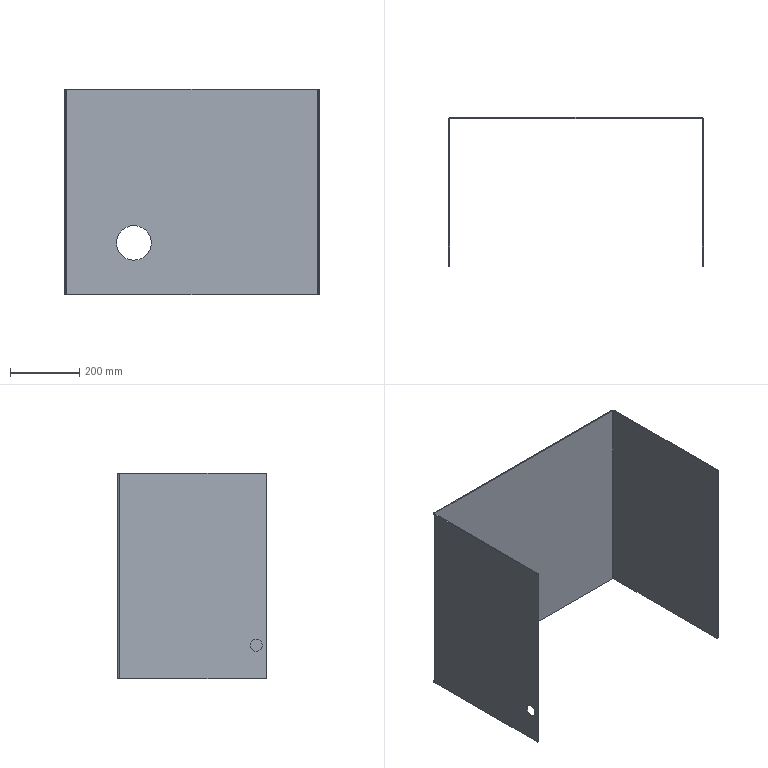Part | SolidWorks | features ICE 3, FlatPattern 1, SMBaseFlange 1, SheetMetal 1 | 1 solid | 30 faces | box 736 x 430 x 594 mm | volume 2800017 mm3 | plane 18 | cylinder 12 | commonest cylinder face diameters 7 x4 6 x2 12 x2 35 x2 100 x2
STEP:
#1=CARTESIAN_POINT('',(200.,427.,100.));
#2=VERTEX_POINT('',#1);
#3=CARTESIAN_POINT('',(200.,427.,200.));
#4=VERTEX_POINT('',#3);
#5=CARTESIAN_POINT('',(200.,427.,150.));
#6=DIRECTION('',(0.,1.,0.));
#7=DIRECTION('',(0.,0.,1.));
#8=AXIS2_PLACEMENT_3D('',#5,#6,#7);
#9=CIRCLE('',#8,50.);
#10=EDGE_CURVE('',#2,#4,#9,.T.);
#11=ORIENTED_EDGE('',*,*,#10,.F.);
#12=CARTESIAN_POINT('',(200.,430.,100.));
#13=VERTEX_POINT('',#12);
#14=CARTESIAN_POINT('',(200.,420.,100.));
#15=DIRECTION('',(0.,1.,0.));
#16=VECTOR('',#15,1000.);
#17=LINE('',#14,#16);
#18=EDGE_CURVE('',#2,#13,#17,.T.);
#19=ORIENTED_EDGE('',*,*,#18,.T.);
#20=CARTESIAN_POINT('',(200.,430.,200.));
#21=VERTEX_POINT('',#20);
#22=CARTESIAN_POINT('',(200.,430.,150.));
#23=DIRECTION('',(0.,1.,0.));
#24=DIRECTION('',(0.,0.,1.));
#25=AXIS2_PLACEMENT_3D('',#22,#23,#24);
#26=CIRCLE('',#25,50.);
#27=EDGE_CURVE('',#13,#21,#26,.T.);
#28=ORIENTED_EDGE('',*,*,#27,.T.);
#29=CARTESIAN_POINT('',(200.,420.,200.));
#30=DIRECTION('',(0.,1.,0.));
#31=VECTOR('',#30,1000.);
#32=LINE('',#29,#31);
#33=EDGE_CURVE('',#4,#21,#32,.T.);
#34=ORIENTED_EDGE('',*,*,#33,.F.);
#35=EDGE_LOOP('',(#11,#19,#28,#34));
#36=FACE_OUTER_BOUND('',#35,.T.);
#37=CARTESIAN_POINT('',(200.,420.,150.));
#38=DIRECTION('',(0.,1.,0.));
#39=DIRECTION('',(0.,0.,1.));
#40=AXIS2_PLACEMENT_3D('',#37,#38,#39);
#41=CYLINDRICAL_SURFACE('',#40,50.);
#42=ADVANCED_FACE('',(#36),#41,.F.);
#43=CARTESIAN_POINT('',(3.,30.,79.5));
#44=VERTEX_POINT('',#43);
#45=CARTESIAN_POINT('',(3.,30.,114.5));
#46=VERTEX_POINT('',#45);
#47=CARTESIAN_POINT('',(3.,30.,97.));
#48=DIRECTION('',(-1.,0.,0.));
#49=DIRECTION('',(0.,0.,1.));
#50=AXIS2_PLACEMENT_3D('',#47,#48,#49);
#51=CIRCLE('',#50,17.5);
#52=EDGE_CURVE('',#44,#46,#51,.T.);
#53=ORIENTED_EDGE('',*,*,#52,.F.);
#54=CARTESIAN_POINT('',(0.,30.,79.5));
#55=VERTEX_POINT('',#54);
#56=CARTESIAN_POINT('',(10.,30.,79.5));
#57=DIRECTION('',(-1.,0.,0.));
#58=VECTOR('',#57,1000.);
#59=LINE('',#56,#58);
#60=EDGE_CURVE('',#44,#55,#59,.T.);
#61=ORIENTED_EDGE('',*,*,#60,.T.);
#62=CARTESIAN_POINT('',(0.,30.,114.5));
#63=VERTEX_POINT('',#62);
#64=CARTESIAN_POINT('',(0.,30.,97.));
#65=DIRECTION('',(-1.,0.,0.));
#66=DIRECTION('',(0.,0.,1.));
#67=AXIS2_PLACEMENT_3D('',#64,#65,#66);
#68=CIRCLE('',#67,17.5);
#69=EDGE_CURVE('',#55,#63,#68,.T.);
#70=ORIENTED_EDGE('',*,*,#69,.T.);
#71=CARTESIAN_POINT('',(10.,30.,114.5));
#72=DIRECTION('',(-1.,0.,0.));
#73=VECTOR('',#72,1000.);
#74=LINE('',#71,#73);
#75=EDGE_CURVE('',#46,#63,#74,.T.);
#76=ORIENTED_EDGE('',*,*,#75,.F.);
#77=EDGE_LOOP('',(#53,#61,#70,#76));
#78=FACE_OUTER_BOUND('',#77,.T.);
#79=CARTESIAN_POINT('',(10.,30.,97.));
#80=DIRECTION('',(-1.,0.,0.));
#81=DIRECTION('',(0.,0.,1.));
#82=AXIS2_PLACEMENT_3D('',#79,#80,#81);
#83=CYLINDRICAL_SURFACE('',#82,17.5);
#84=ADVANCED_FACE('',(#78),#83,.F.);
#85=CARTESIAN_POINT('',(733.,0.,590.5));
#86=VERTEX_POINT('',#85);
#87=CARTESIAN_POINT('',(733.,3.5,594.));
#88=VERTEX_POINT('',#87);
#89=CARTESIAN_POINT('',(733.,3.5,590.5));
#90=DIRECTION('',(-1.,0.,0.));
#91=DIRECTION('',(0.,0.,-1.));
#92=AXIS2_PLACEMENT_3D('',#89,#90,#91);
#93=CIRCLE('',#92,3.5);
#94=EDGE_CURVE('',#86,#88,#93,.T.);
#95=ORIENTED_EDGE('',*,*,#94,.T.);
#96=CARTESIAN_POINT('',(733.,424.,594.));
#97=VERTEX_POINT('',#96);
#98=CARTESIAN_POINT('',(733.,430.,594.));
#99=DIRECTION('',(0.,-1.,0.));
#100=VECTOR('',#99,1000.);
#101=LINE('',#98,#100);
#102=EDGE_CURVE('',#97,#88,#101,.T.);
#103=ORIENTED_EDGE('',*,*,#102,.F.);
#104=CARTESIAN_POINT('',(733.,424.,0.));
#105=VERTEX_POINT('',#104);
#106=CARTESIAN_POINT('',(733.,424.,594.));
#107=DIRECTION('',(0.,0.,-1.));
#108=VECTOR('',#107,1000.);
#109=LINE('',#106,#108);
#110=EDGE_CURVE('',#97,#105,#109,.T.);
#111=ORIENTED_EDGE('',*,*,#110,.T.);
#112=CARTESIAN_POINT('',(733.,3.5,0.));
#113=VERTEX_POINT('',#112);
#114=CARTESIAN_POINT('',(733.,430.,0.));
#115=DIRECTION('',(0.,-1.,0.));
#116=VECTOR('',#115,1000.);
#117=LINE('',#114,#116);
#118=EDGE_CURVE('',#105,#113,#117,.T.);
#119=ORIENTED_EDGE('',*,*,#118,.T.);
#120=CARTESIAN_POINT('',(733.,0.,3.5));
#121=VERTEX_POINT('',#120);
#122=CARTESIAN_POINT('',(733.,3.5,3.5));
#123=DIRECTION('',(-1.,0.,0.));
#124=DIRECTION('',(0.,0.,-1.));
#125=AXIS2_PLACEMENT_3D('',#122,#123,#124);
#126=CIRCLE('',#125,3.5);
#127=EDGE_CURVE('',#113,#121,#126,.T.);
#128=ORIENTED_EDGE('',*,*,#127,.T.);
#129=CARTESIAN_POINT('',(733.,0.,594.));
#130=DIRECTION('',(0.,0.,-1.));
#131=VECTOR('',#130,1000.);
#132=LINE('',#129,#131);
#133=EDGE_CURVE('',#86,#121,#132,.T.);
#134=ORIENTED_EDGE('',*,*,#133,.F.);
#135=EDGE_LOOP('',(#95,#103,#111,#119,#128,#134));
#136=FACE_OUTER_BOUND('',#135,.T.);
#137=CARTESIAN_POINT('',(733.,430.,594.));
#138=DIRECTION('',(1.,0.,0.));
#139=DIRECTION('',(0.,0.,-1.));
#140=AXIS2_PLACEMENT_3D('',#137,#138,#139);
#141=PLANE('',#140);
#142=ADVANCED_FACE('',(#136),#141,.F.);
#143=CARTESIAN_POINT('',(736.,424.,594.));
#144=VERTEX_POINT('',#143);
#145=CARTESIAN_POINT('',(736.,3.5,594.));
#146=VERTEX_POINT('',#145);
#147=CARTESIAN_POINT('',(736.,430.,594.));
#148=DIRECTION('',(0.,-1.,0.));
#149=VECTOR('',#148,1000.);
#150=LINE('',#147,#149);
#151=EDGE_CURVE('',#144,#146,#150,.T.);
#152=ORIENTED_EDGE('',*,*,#151,.T.);
#153=CARTESIAN_POINT('',(736.,0.,590.5));
#154=VERTEX_POINT('',#153);
#155=CARTESIAN_POINT('',(736.,3.5,590.5));
#156=DIRECTION('',(-1.,0.,0.));
#157=DIRECTION('',(0.,0.,-1.));
#158=AXIS2_PLACEMENT_3D('',#155,#156,#157);
#159=CIRCLE('',#158,3.5);
#160=EDGE_CURVE('',#154,#146,#159,.T.);
#161=ORIENTED_EDGE('',*,*,#160,.F.);
#162=CARTESIAN_POINT('',(736.,0.,3.5));
#163=VERTEX_POINT('',#162);
#164=CARTESIAN_POINT('',(736.,0.,594.));
#165=DIRECTION('',(0.,0.,-1.));
#166=VECTOR('',#165,1000.);
#167=LINE('',#164,#166);
#168=EDGE_CURVE('',#154,#163,#167,.T.);
#169=ORIENTED_EDGE('',*,*,#168,.T.);
#170=CARTESIAN_POINT('',(736.,3.5,0.));
#171=VERTEX_POINT('',#170);
#172=CARTESIAN_POINT('',(736.,3.5,3.5));
#173=DIRECTION('',(-1.,0.,0.));
#174=DIRECTION('',(0.,0.,-1.));
#175=AXIS2_PLACEMENT_3D('',#172,#173,#174);
#176=CIRCLE('',#175,3.5);
#177=EDGE_CURVE('',#171,#163,#176,.T.);
#178=ORIENTED_EDGE('',*,*,#177,.F.);
#179=CARTESIAN_POINT('',(736.,424.,0.));
#180=VERTEX_POINT('',#179);
#181=CARTESIAN_POINT('',(736.,430.,0.));
#182=DIRECTION('',(0.,-1.,0.));
#183=VECTOR('',#182,1000.);
#184=LINE('',#181,#183);
#185=EDGE_CURVE('',#180,#171,#184,.T.);
#186=ORIENTED_EDGE('',*,*,#185,.F.);
#187=CARTESIAN_POINT('',(736.,424.,594.));
#188=DIRECTION('',(0.,0.,-1.));
#189=VECTOR('',#188,1000.);
#190=LINE('',#187,#189);
#191=EDGE_CURVE('',#144,#180,#190,.T.);
#192=ORIENTED_EDGE('',*,*,#191,.F.);
#193=EDGE_LOOP('',(#152,#161,#169,#178,#186,#192));
#194=FACE_OUTER_BOUND('',#193,.T.);
#195=CARTESIAN_POINT('',(736.,430.,594.));
#196=DIRECTION('',(1.,0.,0.));
#197=DIRECTION('',(0.,0.,-1.));
#198=AXIS2_PLACEMENT_3D('',#195,#196,#197);
#199=PLANE('',#198);
#200=ADVANCED_FACE('',(#194),#199,.T.);
#201=ORIENTED_EDGE('',*,*,#102,.T.);
#202=CARTESIAN_POINT('',(733.,3.5,594.));
#203=DIRECTION('',(1.,0.,0.));
#204=VECTOR('',#203,1000.);
#205=LINE('',#202,#204);
#206=EDGE_CURVE('',#88,#146,#205,.T.);
#207=ORIENTED_EDGE('',*,*,#206,.T.);
#208=ORIENTED_EDGE('',*,*,#151,.F.);
#209=CARTESIAN_POINT('',(736.,424.,594.));
#210=DIRECTION('',(-1.,0.,0.));
#211=VECTOR('',#210,1000.);
#212=LINE('',#209,#211);
#213=EDGE_CURVE('',#144,#97,#212,.T.);
#214=ORIENTED_EDGE('',*,*,#213,.T.);
#215=EDGE_LOOP('',(#201,#207,#208,#214));
#216=FACE_OUTER_BOUND('',#215,.T.);
#217=CARTESIAN_POINT('',(730.,427.,594.));
#218=DIRECTION('',(0.,0.,1.));
#219=DIRECTION('',(1.,0.,0.));
#220=AXIS2_PLACEMENT_3D('',#217,#218,#219);
#221=PLANE('',#220);
#222=ADVANCED_FACE('',(#216),#221,.T.);
#223=CARTESIAN_POINT('',(733.,0.,590.5));
#224=DIRECTION('',(1.,0.,0.));
#225=VECTOR('',#224,1000.);
#226=LINE('',#223,#225);
#227=EDGE_CURVE('',#86,#154,#226,.T.);
#228=ORIENTED_EDGE('',*,*,#227,.F.);
#229=ORIENTED_EDGE('',*,*,#133,.T.);
#230=CARTESIAN_POINT('',(733.,0.,3.5));
#231=DIRECTION('',(1.,0.,0.));
#232=VECTOR('',#231,1000.);
#233=LINE('',#230,#232);
#234=EDGE_CURVE('',#121,#163,#233,.T.);
#235=ORIENTED_EDGE('',*,*,#234,.T.);
#236=ORIENTED_EDGE('',*,*,#168,.F.);
#237=EDGE_LOOP('',(#228,#229,#235,#236));
#238=FACE_OUTER_BOUND('',#237,.T.);
#239=CARTESIAN_POINT('',(736.,0.,594.));
#240=DIRECTION('',(0.,-1.,0.));
#241=DIRECTION('',(0.,0.,-1.));
#242=AXIS2_PLACEMENT_3D('',#239,#240,#241);
#243=PLANE('',#242);
#244=ADVANCED_FACE('',(#238),#243,.T.);
#245=CARTESIAN_POINT('',(733.,3.5,0.));
#246=DIRECTION('',(1.,0.,0.));
#247=VECTOR('',#246,1000.);
#248=LINE('',#245,#247);
#249=EDGE_CURVE('',#113,#171,#248,.T.);
#250=ORIENTED_EDGE('',*,*,#249,.F.);
#251=ORIENTED_EDGE('',*,*,#118,.F.);
#252=CARTESIAN_POINT('',(733.,424.,0.));
#253=DIRECTION('',(1.,0.,0.));
#254=VECTOR('',#253,1000.);
#255=LINE('',#252,#254);
#256=EDGE_CURVE('',#105,#180,#255,.T.);
#257=ORIENTED_EDGE('',*,*,#256,.T.);
#258=ORIENTED_EDGE('',*,*,#185,.T.);
#259=EDGE_LOOP('',(#250,#251,#257,#258));
#260=FACE_OUTER_BOUND('',#259,.T.);
#261=CARTESIAN_POINT('',(730.,424.,0.));
#262=DIRECTION('',(0.,0.,1.));
#263=DIRECTION('',(1.,0.,0.));
#264=AXIS2_PLACEMENT_3D('',#261,#262,#263);
#265=PLANE('',#264);
#266=ADVANCED_FACE('',(#260),#265,.F.);
#267=CARTESIAN_POINT('',(0.,30.,97.));
#268=DIRECTION('',(-1.,0.,0.));
#269=DIRECTION('',(0.,0.,1.));
#270=AXIS2_PLACEMENT_3D('',#267,#268,#269);
#271=CIRCLE('',#270,17.5);
#272=EDGE_CURVE('',#63,#55,#271,.T.);
#273=ORIENTED_EDGE('',*,*,#272,.F.);
#274=ORIENTED_EDGE('',*,*,#69,.F.);
#275=EDGE_LOOP('',(#273,#274));
#276=FACE_BOUND('',#275,.T.);
#277=CARTESIAN_POINT('',(0.,0.,590.5));
#278=VERTEX_POINT('',#277);
#279=CARTESIAN_POINT('',(0.,0.,3.5));
#280=VERTEX_POINT('',#279);
#281=CARTESIAN_POINT('',(0.,0.,594.));
#282=DIRECTION('',(0.,0.,-1.));
#283=VECTOR('',#282,1000.);
#284=LINE('',#281,#283);
#285=EDGE_CURVE('',#278,#280,#284,.T.);
#286=ORIENTED_EDGE('',*,*,#285,.F.);
#287=CARTESIAN_POINT('',(0.,3.5,594.));
#288=VERTEX_POINT('',#287);
#289=CARTESIAN_POINT('',(0.,3.5,590.5));
#290=DIRECTION('',(1.,0.,0.));
#291=DIRECTION('',(0.,0.,1.));
#292=AXIS2_PLACEMENT_3D('',#289,#290,#291);
#293=CIRCLE('',#292,3.5);
#294=EDGE_CURVE('',#288,#278,#293,.T.);
#295=ORIENTED_EDGE('',*,*,#294,.F.);
#296=CARTESIAN_POINT('',(0.,424.,594.));
#297=VERTEX_POINT('',#296);
#298=CARTESIAN_POINT('',(0.,0.,594.));
#299=DIRECTION('',(0.,1.,0.));
#300=VECTOR('',#299,1000.);
#301=LINE('',#298,#300);
#302=EDGE_CURVE('',#288,#297,#301,.T.);
#303=ORIENTED_EDGE('',*,*,#302,.T.);
#304=CARTESIAN_POINT('',(0.,424.,0.));
#305=VERTEX_POINT('',#304);
#306=CARTESIAN_POINT('',(0.,424.,594.));
#307=DIRECTION('',(0.,0.,-1.));
#308=VECTOR('',#307,1000.);
#309=LINE('',#306,#308);
#310=EDGE_CURVE('',#297,#305,#309,.T.);
#311=ORIENTED_EDGE('',*,*,#310,.T.);
#312=CARTESIAN_POINT('',(0.,3.5,0.));
#313=VERTEX_POINT('',#312);
#314=CARTESIAN_POINT('',(0.,0.,0.));
#315=DIRECTION('',(0.,1.,0.));
#316=VECTOR('',#315,1000.);
#317=LINE('',#314,#316);
#318=EDGE_CURVE('',#313,#305,#317,.T.);
#319=ORIENTED_EDGE('',*,*,#318,.F.);
#320=CARTESIAN_POINT('',(0.,3.5,3.5));
#321=DIRECTION('',(1.,0.,0.));
#322=DIRECTION('',(0.,0.,1.));
#323=AXIS2_PLACEMENT_3D('',#320,#321,#322);
#324=CIRCLE('',#323,3.5);
#325=EDGE_CURVE('',#280,#313,#324,.T.);
#326=ORIENTED_EDGE('',*,*,#325,.F.);
#327=EDGE_LOOP('',(#286,#295,#303,#311,#319,#326));
#328=FACE_OUTER_BOUND('',#327,.T.);
#329=CARTESIAN_POINT('',(0.,0.,594.));
#330=DIRECTION('',(-1.,0.,0.));
#331=DIRECTION('',(0.,0.,1.));
#332=AXIS2_PLACEMENT_3D('',#329,#330,#331);
#333=PLANE('',#332);
#334=ADVANCED_FACE('',(#276,#328),#333,.T.);
#335=CARTESIAN_POINT('',(3.,30.,97.));
#336=DIRECTION('',(-1.,0.,0.));
#337=DIRECTION('',(0.,0.,1.));
#338=AXIS2_PLACEMENT_3D('',#335,#336,#337);
#339=CIRCLE('',#338,17.5);
#340=EDGE_CURVE('',#46,#44,#339,.T.);
#341=ORIENTED_EDGE('',*,*,#340,.T.);
#342=ORIENTED_EDGE('',*,*,#52,.T.);
#343=EDGE_LOOP('',(#341,#342));
#344=FACE_BOUND('',#343,.T.);
#345=CARTESIAN_POINT('',(3.,3.5,594.));
#346=VERTEX_POINT('',#345);
#347=CARTESIAN_POINT('',(3.,0.,590.5));
#348=VERTEX_POINT('',#347);
#349=CARTESIAN_POINT('',(3.,3.5,590.5));
#350=DIRECTION('',(1.,0.,0.));
#351=DIRECTION('',(0.,0.,1.));
#352=AXIS2_PLACEMENT_3D('',#349,#350,#351);
#353=CIRCLE('',#352,3.5);
#354=EDGE_CURVE('',#346,#348,#353,.T.);
#355=ORIENTED_EDGE('',*,*,#354,.T.);
#356=CARTESIAN_POINT('',(3.,0.,3.5));
#357=VERTEX_POINT('',#356);
#358=CARTESIAN_POINT('',(3.,0.,594.));
#359=DIRECTION('',(0.,0.,-1.));
#360=VECTOR('',#359,1000.);
#361=LINE('',#358,#360);
#362=EDGE_CURVE('',#348,#357,#361,.T.);
#363=ORIENTED_EDGE('',*,*,#362,.T.);
#364=CARTESIAN_POINT('',(3.,3.5,0.));
#365=VERTEX_POINT('',#364);
#366=CARTESIAN_POINT('',(3.,3.5,3.5));
#367=DIRECTION('',(1.,0.,0.));
#368=DIRECTION('',(0.,0.,1.));
#369=AXIS2_PLACEMENT_3D('',#366,#367,#368);
#370=CIRCLE('',#369,3.5);
#371=EDGE_CURVE('',#357,#365,#370,.T.);
#372=ORIENTED_EDGE('',*,*,#371,.T.);
#373=CARTESIAN_POINT('',(3.,424.,0.));
#374=VERTEX_POINT('',#373);
#375=CARTESIAN_POINT('',(3.,0.,0.));
#376=DIRECTION('',(0.,1.,0.));
#377=VECTOR('',#376,1000.);
#378=LINE('',#375,#377);
#379=EDGE_CURVE('',#365,#374,#378,.T.);
#380=ORIENTED_EDGE('',*,*,#379,.T.);
#381=CARTESIAN_POINT('',(3.,424.,594.));
#382=VERTEX_POINT('',#381);
#383=CARTESIAN_POINT('',(3.,424.,594.));
#384=DIRECTION('',(0.,0.,-1.));
#385=VECTOR('',#384,1000.);
#386=LINE('',#383,#385);
#387=EDGE_CURVE('',#382,#374,#386,.T.);
#388=ORIENTED_EDGE('',*,*,#387,.F.);
#389=CARTESIAN_POINT('',(3.,0.,594.));
#390=DIRECTION('',(0.,1.,0.));
#391=VECTOR('',#390,1000.);
#392=LINE('',#389,#391);
#393=EDGE_CURVE('',#346,#382,#392,.T.);
#394=ORIENTED_EDGE('',*,*,#393,.F.);
#395=EDGE_LOOP('',(#355,#363,#372,#380,#388,#394));
#396=FACE_OUTER_BOUND('',#395,.T.);
#397=CARTESIAN_POINT('',(3.,0.,594.));
#398=DIRECTION('',(-1.,0.,0.));
#399=DIRECTION('',(0.,0.,1.));
#400=AXIS2_PLACEMENT_3D('',#397,#398,#399);
#401=PLANE('',#400);
#402=ADVANCED_FACE('',(#344,#396),#401,.F.);
#403=ORIENTED_EDGE('',*,*,#362,.F.);
#404=CARTESIAN_POINT('',(3.,0.,590.5));
#405=DIRECTION('',(-1.,0.,0.));
#406=VECTOR('',#405,1000.);
#407=LINE('',#404,#406);
#408=EDGE_CURVE('',#348,#278,#407,.T.);
#409=ORIENTED_EDGE('',*,*,#408,.T.);
#410=ORIENTED_EDGE('',*,*,#285,.T.);
#411=CARTESIAN_POINT('',(3.,0.,3.5));
#412=DIRECTION('',(-1.,0.,0.));
#413=VECTOR('',#412,1000.);
#414=LINE('',#411,#413);
#415=EDGE_CURVE('',#357,#280,#414,.T.);
#416=ORIENTED_EDGE('',*,*,#415,.F.);
#417=EDGE_LOOP('',(#403,#409,#410,#416));
#418=FACE_OUTER_BOUND('',#417,.T.);
#419=CARTESIAN_POINT('',(3.,0.,594.));
#420=DIRECTION('',(0.,-1.,0.));
#421=DIRECTION('',(0.,0.,-1.));
#422=AXIS2_PLACEMENT_3D('',#419,#420,#421);
#423=PLANE('',#422);
#424=ADVANCED_FACE('',(#418),#423,.T.);
#425=ORIENTED_EDGE('',*,*,#379,.F.);
#426=CARTESIAN_POINT('',(3.,3.5,0.));
#427=DIRECTION('',(-1.,0.,0.));
#428=VECTOR('',#427,1000.);
#429=LINE('',#426,#428);
#430=EDGE_CURVE('',#365,#313,#429,.T.);
#431=ORIENTED_EDGE('',*,*,#430,.T.);
#432=ORIENTED_EDGE('',*,*,#318,.T.);
#433=CARTESIAN_POINT('',(0.,424.,0.));
#434=DIRECTION('',(1.,0.,0.));
#435=VECTOR('',#434,1000.);
#436=LINE('',#433,#435);
#437=EDGE_CURVE('',#305,#374,#436,.T.);
#438=ORIENTED_EDGE('',*,*,#437,.T.);
#439=EDGE_LOOP('',(#425,#431,#432,#438));
#440=FACE_OUTER_BOUND('',#439,.T.);
#441=CARTESIAN_POINT('',(6.,427.,0.));
#442=DIRECTION('',(0.,0.,-1.));
#443=DIRECTION('',(-1.,0.,0.));
#444=AXIS2_PLACEMENT_3D('',#441,#442,#443);
#445=PLANE('',#444);
#446=ADVANCED_FACE('',(#440),#445,.T.);
#447=CARTESIAN_POINT('',(6.,430.,594.));
#448=VERTEX_POINT('',#447);
#449=CARTESIAN_POINT('',(6.,427.,594.));
#450=VERTEX_POINT('',#449);
#451=CARTESIAN_POINT('',(6.,430.,594.));
#452=DIRECTION('',(0.,-1.,0.));
#453=VECTOR('',#452,1000.);
#454=LINE('',#451,#453);
#455=EDGE_CURVE('',#448,#450,#454,.T.);
#456=ORIENTED_EDGE('',*,*,#455,.F.);
#457=CARTESIAN_POINT('',(6.,424.,594.));
#458=DIRECTION('',(0.,0.,-1.));
#459=DIRECTION('',(1.,0.,0.));
#460=AXIS2_PLACEMENT_3D('',#457,#458,#459);
#461=CIRCLE('',#460,6.);
#462=EDGE_CURVE('',#297,#448,#461,.T.);
#463=ORIENTED_EDGE('',*,*,#462,.F.);
#464=CARTESIAN_POINT('',(3.,424.,594.));
#465=DIRECTION('',(-1.,0.,0.));
#466=VECTOR('',#465,1000.);
#467=LINE('',#464,#466);
#468=EDGE_CURVE('',#382,#297,#467,.T.);
#469=ORIENTED_EDGE('',*,*,#468,.F.);
#470=CARTESIAN_POINT('',(6.,424.,594.));
#471=DIRECTION('',(0.,0.,-1.));
#472=DIRECTION('',(1.,0.,0.));
#473=AXIS2_PLACEMENT_3D('',#470,#471,#472);
#474=CIRCLE('',#473,3.);
#475=EDGE_CURVE('',#382,#450,#474,.T.);
#476=ORIENTED_EDGE('',*,*,#475,.T.);
#477=EDGE_LOOP('',(#456,#463,#469,#476));
#478=FACE_OUTER_BOUND('',#477,.T.);
#479=CARTESIAN_POINT('',(6.,430.,594.));
#480=DIRECTION('',(0.,0.,1.));
#481=DIRECTION('',(1.,0.,0.));
#482=AXIS2_PLACEMENT_3D('',#479,#480,#481);
#483=PLANE('',#482);
#484=ADVANCED_FACE('',(#478),#483,.T.);
#485=CARTESIAN_POINT('',(730.,430.,594.));
#486=VERTEX_POINT('',#485);
#487=CARTESIAN_POINT('',(0.,430.,594.));
#488=DIRECTION('',(1.,0.,0.));
#489=VECTOR('',#488,1000.);
#490=LINE('',#487,#489);
#491=EDGE_CURVE('',#448,#486,#490,.T.);
#492=ORIENTED_EDGE('',*,*,#491,.F.);
#493=ORIENTED_EDGE('',*,*,#455,.T.);
#494=CARTESIAN_POINT('',(730.,427.,594.));
#495=VERTEX_POINT('',#494);
#496=CARTESIAN_POINT('',(0.,427.,594.));
#497=DIRECTION('',(1.,0.,0.));
#498=VECTOR('',#497,1000.);
#499=LINE('',#496,#498);
#500=EDGE_CURVE('',#450,#495,#499,.T.);
#501=ORIENTED_EDGE('',*,*,#500,.T.);
#502=CARTESIAN_POINT('',(730.,427.,594.));
#503=DIRECTION('',(0.,1.,0.));
#504=VECTOR('',#503,1000.);
#505=LINE('',#502,#504);
#506=EDGE_CURVE('',#495,#486,#505,.T.);
#507=ORIENTED_EDGE('',*,*,#506,.T.);
#508=EDGE_LOOP('',(#492,#493,#501,#507));
#509=FACE_OUTER_BOUND('',#508,.T.);
#510=CARTESIAN_POINT('',(3.,424.,594.));
#511=DIRECTION('',(0.,0.,1.));
#512=DIRECTION('',(1.,0.,0.));
#513=AXIS2_PLACEMENT_3D('',#510,#511,#512);
#514=PLANE('',#513);
#515=ADVANCED_FACE('',(#509),#514,.T.);
#516=ORIENTED_EDGE('',*,*,#437,.F.);
#517=CARTESIAN_POINT('',(6.,430.,0.));
#518=VERTEX_POINT('',#517);
#519=CARTESIAN_POINT('',(6.,424.,0.));
#520=DIRECTION('',(0.,0.,-1.));
#521=DIRECTION('',(1.,0.,0.));
#522=AXIS2_PLACEMENT_3D('',#519,#520,#521);
#523=CIRCLE('',#522,6.);
#524=EDGE_CURVE('',#305,#518,#523,.T.);
#525=ORIENTED_EDGE('',*,*,#524,.T.);
#526=CARTESIAN_POINT('',(6.,427.,0.));
#527=VERTEX_POINT('',#526);
#528=CARTESIAN_POINT('',(6.,427.,0.));
#529=DIRECTION('',(0.,1.,0.));
#530=VECTOR('',#529,1000.);
#531=LINE('',#528,#530);
#532=EDGE_CURVE('',#527,#518,#531,.T.);
#533=ORIENTED_EDGE('',*,*,#532,.F.);
#534=CARTESIAN_POINT('',(6.,424.,0.));
#535=DIRECTION('',(0.,0.,-1.));
#536=DIRECTION('',(1.,0.,0.));
#537=AXIS2_PLACEMENT_3D('',#534,#535,#536);
#538=CIRCLE('',#537,3.);
#539=EDGE_CURVE('',#374,#527,#538,.T.);
#540=ORIENTED_EDGE('',*,*,#539,.F.);
#541=EDGE_LOOP('',(#516,#525,#533,#540));
#542=FACE_OUTER_BOUND('',#541,.T.);
#543=CARTESIAN_POINT('',(0.,424.,0.));
#544=DIRECTION('',(0.,0.,-1.));
#545=DIRECTION('',(-1.,0.,0.));
#546=AXIS2_PLACEMENT_3D('',#543,#544,#545);
#547=PLANE('',#546);
#548=ADVANCED_FACE('',(#542),#547,.T.);
#549=ORIENTED_EDGE('',*,*,#213,.F.);
#550=CARTESIAN_POINT('',(730.,424.,594.));
#551=DIRECTION('',(0.,0.,-1.));
#552=DIRECTION('',(1.,0.,0.));
#553=AXIS2_PLACEMENT_3D('',#550,#551,#552);
#554=CIRCLE('',#553,6.);
#555=EDGE_CURVE('',#486,#144,#554,.T.);
#556=ORIENTED_EDGE('',*,*,#555,.F.);
#557=ORIENTED_EDGE('',*,*,#506,.F.);
#558=CARTESIAN_POINT('',(730.,424.,594.));
#559=DIRECTION('',(0.,0.,-1.));
#560=DIRECTION('',(1.,0.,0.));
#561=AXIS2_PLACEMENT_3D('',#558,#559,#560);
#562=CIRCLE('',#561,3.);
#563=EDGE_CURVE('',#495,#97,#562,.T.);
#564=ORIENTED_EDGE('',*,*,#563,.T.);
#565=EDGE_LOOP('',(#549,#556,#557,#564));
#566=FACE_OUTER_BOUND('',#565,.T.);
#567=CARTESIAN_POINT('',(736.,424.,594.));
#568=DIRECTION('',(0.,0.,1.));
#569=DIRECTION('',(1.,0.,0.));
#570=AXIS2_PLACEMENT_3D('',#567,#568,#569);
#571=PLANE('',#570);
#572=ADVANCED_FACE('',(#566),#571,.T.);
#573=CARTESIAN_POINT('',(730.,430.,0.));
#574=VERTEX_POINT('',#573);
#575=CARTESIAN_POINT('',(730.,427.,0.));
#576=VERTEX_POINT('',#575);
#577=CARTESIAN_POINT('',(730.,430.,0.));
#578=DIRECTION('',(0.,-1.,0.));
#579=VECTOR('',#578,1000.);
#580=LINE('',#577,#579);
#581=EDGE_CURVE('',#574,#576,#580,.T.);
#582=ORIENTED_EDGE('',*,*,#581,.F.);
#583=CARTESIAN_POINT('',(730.,424.,0.));
#584=DIRECTION('',(0.,0.,-1.));
#585=DIRECTION('',(1.,0.,0.));
#586=AXIS2_PLACEMENT_3D('',#583,#584,#585);
#587=CIRCLE('',#586,6.);
#588=EDGE_CURVE('',#574,#180,#587,.T.);
#589=ORIENTED_EDGE('',*,*,#588,.T.);
#590=ORIENTED_EDGE('',*,*,#256,.F.);
#591=CARTESIAN_POINT('',(730.,424.,0.));
#592=DIRECTION('',(0.,0.,-1.));
#593=DIRECTION('',(1.,0.,0.));
#594=AXIS2_PLACEMENT_3D('',#591,#592,#593);
#595=CIRCLE('',#594,3.);
#596=EDGE_CURVE('',#576,#105,#595,.T.);
#597=ORIENTED_EDGE('',*,*,#596,.F.);
#598=EDGE_LOOP('',(#582,#589,#590,#597));
#599=FACE_OUTER_BOUND('',#598,.T.);
#600=CARTESIAN_POINT('',(730.,430.,0.));
#601=DIRECTION('',(0.,0.,-1.));
#602=DIRECTION('',(-1.,0.,0.));
#603=AXIS2_PLACEMENT_3D('',#600,#601,#602);
#604=PLANE('',#603);
#605=ADVANCED_FACE('',(#599),#604,.T.);
#606=CARTESIAN_POINT('',(0.,430.,0.));
#607=DIRECTION('',(1.,0.,0.));
#608=VECTOR('',#607,1000.);
#609=LINE('',#606,#608);
#610=EDGE_CURVE('',#518,#574,#609,.T.);
#611=ORIENTED_EDGE('',*,*,#610,.T.);
#612=ORIENTED_EDGE('',*,*,#581,.T.);
#613=CARTESIAN_POINT('',(0.,427.,0.));
#614=DIRECTION('',(1.,0.,0.));
#615=VECTOR('',#614,1000.);
#616=LINE('',#613,#615);
#617=EDGE_CURVE('',#527,#576,#616,.T.);
#618=ORIENTED_EDGE('',*,*,#617,.F.);
#619=ORIENTED_EDGE('',*,*,#532,.T.);
#620=EDGE_LOOP('',(#611,#612,#618,#619));
#621=FACE_OUTER_BOUND('',#620,.T.);
#622=CARTESIAN_POINT('',(733.,424.,0.));
#623=DIRECTION('',(0.,0.,-1.));
#624=DIRECTION('',(-1.,0.,0.));
#625=AXIS2_PLACEMENT_3D('',#622,#623,#624);
#626=PLANE('',#625);
#627=ADVANCED_FACE('',(#621),#626,.T.);
#628=ORIENTED_EDGE('',*,*,#588,.F.);
#629=CARTESIAN_POINT('',(730.,430.,594.));
#630=DIRECTION('',(0.,0.,-1.));
#631=VECTOR('',#630,1000.);
#632=LINE('',#629,#631);
#633=EDGE_CURVE('',#486,#574,#632,.T.);
#634=ORIENTED_EDGE('',*,*,#633,.F.);
#635=ORIENTED_EDGE('',*,*,#555,.T.);
#636=ORIENTED_EDGE('',*,*,#191,.T.);
#637=EDGE_LOOP('',(#628,#634,#635,#636));
#638=FACE_OUTER_BOUND('',#637,.T.);
#639=CARTESIAN_POINT('',(730.,424.,594.));
#640=DIRECTION('',(0.,0.,-1.));
#641=DIRECTION('',(-1.,0.,0.));
#642=AXIS2_PLACEMENT_3D('',#639,#640,#641);
#643=CYLINDRICAL_SURFACE('',#642,6.);
#644=ADVANCED_FACE('',(#638),#643,.T.);
#645=CARTESIAN_POINT('',(200.,430.,150.));
#646=DIRECTION('',(0.,1.,0.));
#647=DIRECTION('',(0.,0.,1.));
#648=AXIS2_PLACEMENT_3D('',#645,#646,#647);
#649=CIRCLE('',#648,50.);
#650=EDGE_CURVE('',#21,#13,#649,.T.);
#651=ORIENTED_EDGE('',*,*,#650,.F.);
#652=ORIENTED_EDGE('',*,*,#27,.F.);
#653=EDGE_LOOP('',(#651,#652));
#654=FACE_BOUND('',#653,.T.);
#655=ORIENTED_EDGE('',*,*,#610,.F.);
#656=CARTESIAN_POINT('',(6.,430.,594.));
#657=DIRECTION('',(0.,0.,-1.));
#658=VECTOR('',#657,1000.);
#659=LINE('',#656,#658);
#660=EDGE_CURVE('',#448,#518,#659,.T.);
#661=ORIENTED_EDGE('',*,*,#660,.F.);
#662=ORIENTED_EDGE('',*,*,#491,.T.);
#663=ORIENTED_EDGE('',*,*,#633,.T.);
#664=EDGE_LOOP('',(#655,#661,#662,#663));
#665=FACE_OUTER_BOUND('',#664,.T.);
#666=CARTESIAN_POINT('',(0.,430.,594.));
#667=DIRECTION('',(0.,1.,0.));
#668=DIRECTION('',(0.,0.,1.));
#669=AXIS2_PLACEMENT_3D('',#666,#667,#668);
#670=PLANE('',#669);
#671=ADVANCED_FACE('',(#654,#665),#670,.T.);
#672=ORIENTED_EDGE('',*,*,#524,.F.);
#673=ORIENTED_EDGE('',*,*,#310,.F.);
#674=ORIENTED_EDGE('',*,*,#462,.T.);
#675=ORIENTED_EDGE('',*,*,#660,.T.);
#676=EDGE_LOOP('',(#672,#673,#674,#675));
#677=FACE_OUTER_BOUND('',#676,.T.);
#678=CARTESIAN_POINT('',(6.,424.,594.));
#679=DIRECTION('',(0.,0.,-1.));
#680=DIRECTION('',(-1.,0.,0.));
#681=AXIS2_PLACEMENT_3D('',#678,#679,#680);
#682=CYLINDRICAL_SURFACE('',#681,6.);
#683=ADVANCED_FACE('',(#677),#682,.T.);
#684=ORIENTED_EDGE('',*,*,#539,.T.);
#685=CARTESIAN_POINT('',(6.,427.,594.));
#686=DIRECTION('',(0.,0.,-1.));
#687=VECTOR('',#686,1000.);
#688=LINE('',#685,#687);
#689=EDGE_CURVE('',#450,#527,#688,.T.);
#690=ORIENTED_EDGE('',*,*,#689,.F.);
#691=ORIENTED_EDGE('',*,*,#475,.F.);
#692=ORIENTED_EDGE('',*,*,#387,.T.);
#693=EDGE_LOOP('',(#684,#690,#691,#692));
#694=FACE_OUTER_BOUND('',#693,.T.);
#695=CARTESIAN_POINT('',(6.,424.,594.));
#696=DIRECTION('',(0.,0.,-1.));
#697=DIRECTION('',(-1.,0.,0.));
#698=AXIS2_PLACEMENT_3D('',#695,#696,#697);
#699=CYLINDRICAL_SURFACE('',#698,3.);
#700=ADVANCED_FACE('',(#694),#699,.F.);
#701=CARTESIAN_POINT('',(200.,427.,150.));
#702=DIRECTION('',(0.,1.,0.));
#703=DIRECTION('',(0.,0.,1.));
#704=AXIS2_PLACEMENT_3D('',#701,#702,#703);
#705=CIRCLE('',#704,50.);
#706=EDGE_CURVE('',#4,#2,#705,.T.);
#707=ORIENTED_EDGE('',*,*,#706,.T.);
#708=ORIENTED_EDGE('',*,*,#10,.T.);
#709=EDGE_LOOP('',(#707,#708));
#710=FACE_BOUND('',#709,.T.);
#711=ORIENTED_EDGE('',*,*,#617,.T.);
#712=CARTESIAN_POINT('',(730.,427.,594.));
#713=DIRECTION('',(0.,0.,-1.));
#714=VECTOR('',#713,1000.);
#715=LINE('',#712,#714);
#716=EDGE_CURVE('',#495,#576,#715,.T.);
#717=ORIENTED_EDGE('',*,*,#716,.F.);
#718=ORIENTED_EDGE('',*,*,#500,.F.);
#719=ORIENTED_EDGE('',*,*,#689,.T.);
#720=EDGE_LOOP('',(#711,#717,#718,#719));
#721=FACE_OUTER_BOUND('',#720,.T.);
#722=CARTESIAN_POINT('',(0.,427.,594.));
#723=DIRECTION('',(0.,1.,0.));
#724=DIRECTION('',(0.,0.,1.));
#725=AXIS2_PLACEMENT_3D('',#722,#723,#724);
#726=PLANE('',#725);
#727=ADVANCED_FACE('',(#710,#721),#726,.F.);
#728=ORIENTED_EDGE('',*,*,#596,.T.);
#729=ORIENTED_EDGE('',*,*,#110,.F.);
#730=ORIENTED_EDGE('',*,*,#563,.F.);
#731=ORIENTED_EDGE('',*,*,#716,.T.);
#732=EDGE_LOOP('',(#728,#729,#730,#731));
#733=FACE_OUTER_BOUND('',#732,.T.);
#734=CARTESIAN_POINT('',(730.,424.,594.));
#735=DIRECTION('',(0.,0.,-1.));
#736=DIRECTION('',(-1.,0.,0.));
#737=AXIS2_PLACEMENT_3D('',#734,#735,#736);
#738=CYLINDRICAL_SURFACE('',#737,3.);
#739=ADVANCED_FACE('',(#733),#738,.F.);
#740=CARTESIAN_POINT('',(3.,3.5,594.));
#741=DIRECTION('',(-1.,0.,0.));
#742=VECTOR('',#741,1000.);
#743=LINE('',#740,#742);
#744=EDGE_CURVE('',#346,#288,#743,.T.);
#745=ORIENTED_EDGE('',*,*,#744,.F.);
#746=ORIENTED_EDGE('',*,*,#393,.T.);
#747=ORIENTED_EDGE('',*,*,#468,.T.);
#748=ORIENTED_EDGE('',*,*,#302,.F.);
#749=EDGE_LOOP('',(#745,#746,#747,#748));
#750=FACE_OUTER_BOUND('',#749,.T.);
#751=CARTESIAN_POINT('',(730.,424.,594.));
#752=DIRECTION('',(0.,0.,1.));
#753=DIRECTION('',(1.,0.,0.));
#754=AXIS2_PLACEMENT_3D('',#751,#752,#753);
#755=PLANE('',#754);
#756=ADVANCED_FACE('',(#750),#755,.T.);
#757=ORIENTED_EDGE('',*,*,#60,.F.);
#758=ORIENTED_EDGE('',*,*,#340,.F.);
#759=ORIENTED_EDGE('',*,*,#75,.T.);
#760=ORIENTED_EDGE('',*,*,#272,.T.);
#761=EDGE_LOOP('',(#757,#758,#759,#760));
#762=FACE_OUTER_BOUND('',#761,.T.);
#763=CARTESIAN_POINT('',(10.,30.,97.));
#764=DIRECTION('',(-1.,0.,0.));
#765=DIRECTION('',(0.,0.,1.));
#766=AXIS2_PLACEMENT_3D('',#763,#764,#765);
#767=CYLINDRICAL_SURFACE('',#766,17.5);
#768=ADVANCED_FACE('',(#762),#767,.F.);
#769=ORIENTED_EDGE('',*,*,#18,.F.);
#770=ORIENTED_EDGE('',*,*,#706,.F.);
#771=ORIENTED_EDGE('',*,*,#33,.T.);
#772=ORIENTED_EDGE('',*,*,#650,.T.);
#773=EDGE_LOOP('',(#769,#770,#771,#772));
#774=FACE_OUTER_BOUND('',#773,.T.);
#775=CARTESIAN_POINT('',(200.,420.,150.));
#776=DIRECTION('',(0.,1.,0.));
#777=DIRECTION('',(0.,0.,1.));
#778=AXIS2_PLACEMENT_3D('',#775,#776,#777);
#779=CYLINDRICAL_SURFACE('',#778,50.);
#780=ADVANCED_FACE('',(#774),#779,.F.);
#781=ORIENTED_EDGE('',*,*,#430,.F.);
#782=ORIENTED_EDGE('',*,*,#371,.F.);
#783=ORIENTED_EDGE('',*,*,#415,.T.);
#784=ORIENTED_EDGE('',*,*,#325,.T.);
#785=EDGE_LOOP('',(#781,#782,#783,#784));
#786=FACE_OUTER_BOUND('',#785,.T.);
#787=CARTESIAN_POINT('',(3.,3.5,3.5));
#788=DIRECTION('',(-1.,0.,0.));
#789=DIRECTION('',(0.,0.,1.));
#790=AXIS2_PLACEMENT_3D('',#787,#788,#789);
#791=CYLINDRICAL_SURFACE('',#790,3.5);
#792=ADVANCED_FACE('',(#786),#791,.T.);
#793=ORIENTED_EDGE('',*,*,#408,.F.);
#794=ORIENTED_EDGE('',*,*,#354,.F.);
#795=ORIENTED_EDGE('',*,*,#744,.T.);
#796=ORIENTED_EDGE('',*,*,#294,.T.);
#797=EDGE_LOOP('',(#793,#794,#795,#796));
#798=FACE_OUTER_BOUND('',#797,.T.);
#799=CARTESIAN_POINT('',(3.,3.5,590.5));
#800=DIRECTION('',(-1.,0.,0.));
#801=DIRECTION('',(0.,0.,1.));
#802=AXIS2_PLACEMENT_3D('',#799,#800,#801);
#803=CYLINDRICAL_SURFACE('',#802,3.5);
#804=ADVANCED_FACE('',(#798),#803,.T.);
#805=ORIENTED_EDGE('',*,*,#234,.F.);
#806=ORIENTED_EDGE('',*,*,#127,.F.);
#807=ORIENTED_EDGE('',*,*,#249,.T.);
#808=ORIENTED_EDGE('',*,*,#177,.T.);
#809=EDGE_LOOP('',(#805,#806,#807,#808));
#810=FACE_OUTER_BOUND('',#809,.T.);
#811=CARTESIAN_POINT('',(733.,3.5,3.5));
#812=DIRECTION('',(1.,0.,0.));
#813=DIRECTION('',(0.,0.,-1.));
#814=AXIS2_PLACEMENT_3D('',#811,#812,#813);
#815=CYLINDRICAL_SURFACE('',#814,3.5);
#816=ADVANCED_FACE('',(#810),#815,.T.);
#817=ORIENTED_EDGE('',*,*,#206,.F.);
#818=ORIENTED_EDGE('',*,*,#94,.F.);
#819=ORIENTED_EDGE('',*,*,#227,.T.);
#820=ORIENTED_EDGE('',*,*,#160,.T.);
#821=EDGE_LOOP('',(#817,#818,#819,#820));
#822=FACE_OUTER_BOUND('',#821,.T.);
#823=CARTESIAN_POINT('',(733.,3.5,590.5));
#824=DIRECTION('',(1.,0.,0.));
#825=DIRECTION('',(0.,0.,-1.));
#826=AXIS2_PLACEMENT_3D('',#823,#824,#825);
#827=CYLINDRICAL_SURFACE('',#826,3.5);
#828=ADVANCED_FACE('',(#822),#827,.T.);
#829=CLOSED_SHELL('',(#42,#84,#142,#200,#222,#244,#266,#334,#402,#424,#446,#484,#515,#548,#572,#605,#627,#644,#671,#683,#700,#727,#739,#756,#768,#780,#792,#804,#816,#828));
#830=MANIFOLD_SOLID_BREP('',#829);
#831=CARTESIAN_POINT('',(0.,0.,0.));
#832=DIRECTION('',(0.,0.,1.));
#833=DIRECTION('',(1.,0.,0.));
#834=AXIS2_PLACEMENT_3D('',#831,#832,#833);
#835=(LENGTH_UNIT()NAMED_UNIT(*)SI_UNIT(.MILLI.,.METRE.));
#836=UNCERTAINTY_MEASURE_WITH_UNIT(LENGTH_MEASURE(0.00001),#835,'','');
#837=(NAMED_UNIT(*)PLANE_ANGLE_UNIT()SI_UNIT($,.RADIAN.));
#838=(NAMED_UNIT(*)SI_UNIT($,.STERADIAN.)SOLID_ANGLE_UNIT());
#839=(GEOMETRIC_REPRESENTATION_CONTEXT(3)GLOBAL_UNCERTAINTY_ASSIGNED_CONTEXT((#836))GLOBAL_UNIT_ASSIGNED_CONTEXT((#835,#837,#838))REPRESENTATION_CONTEXT('',''));
#840=ADVANCED_BREP_SHAPE_REPRESENTATION('',(#830,#834),#839);